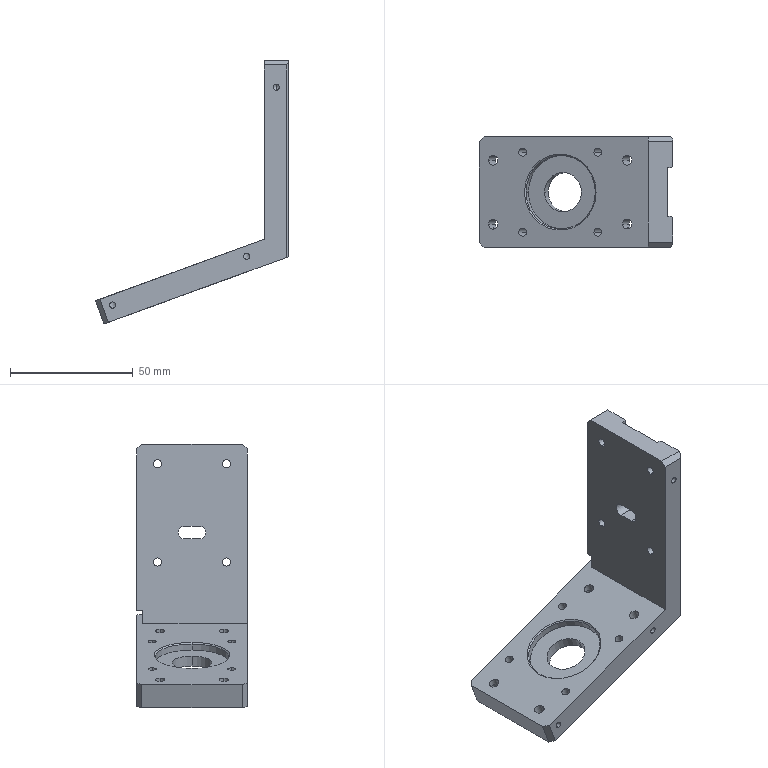Part | SolidWorks | features ICE 8, HoleWzd 6, Chamfer 4, 3DProfileFeature 2, MirrorPattern 2, CirPattern 1, Cut 1, Extrusion 1 | 1 solid | 102 faces | box 78.596 x 45 x 107.362 mm | volume 57483 mm3 | cylinder 58 | plane 32 | cone 12 | commonest cylinder face diameters 3.3 x18 2.5 x16 4 x8 8 x8 5.2 x2 16 x2